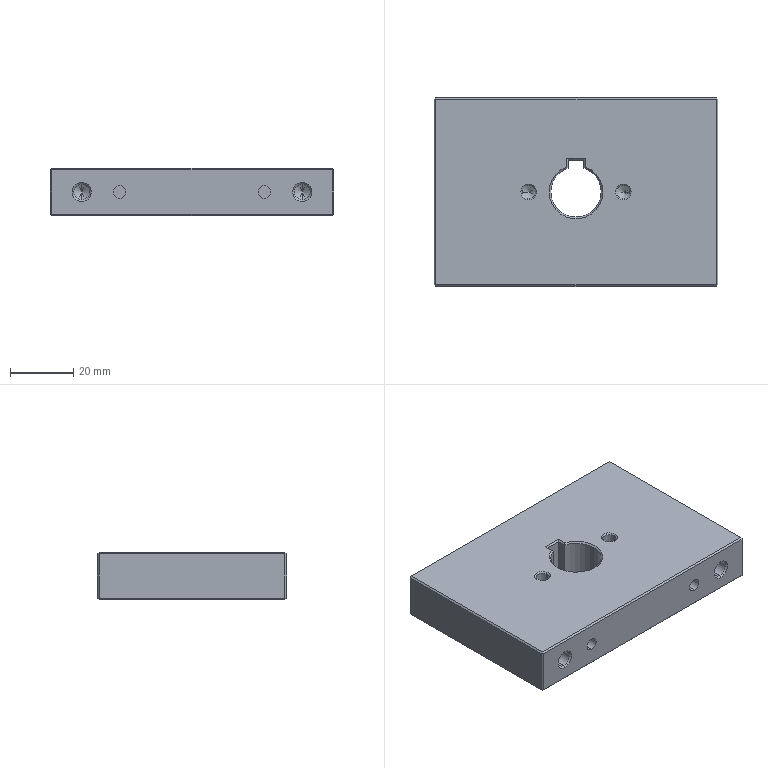Part | SolidWorks | features HoleWzd 3, Chamfer 2, Cut 2, Extrusion 1, ICE 1 | 1 solid | 86 faces | box 90 x 60 x 15 mm | volume 75882 mm3 | plane 37 | cone 30 | cylinder 19 | commonest cylinder face diameters 5 x8 4 x4 4.2 x4 16 x3